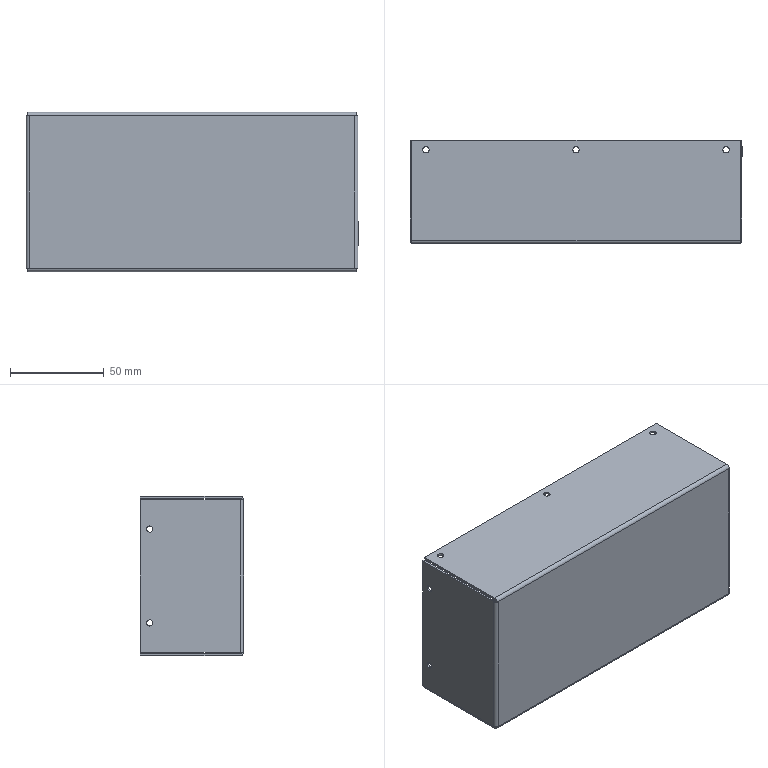Part | SolidWorks | features BaseBody 1 | 1 solid | 54 faces | box 177 x 55 x 85 mm | volume 42380 mm3 | cylinder 28 | plane 26 | commonest cylinder face diameters 3.4 x20 1.473 x4 3.473 x4